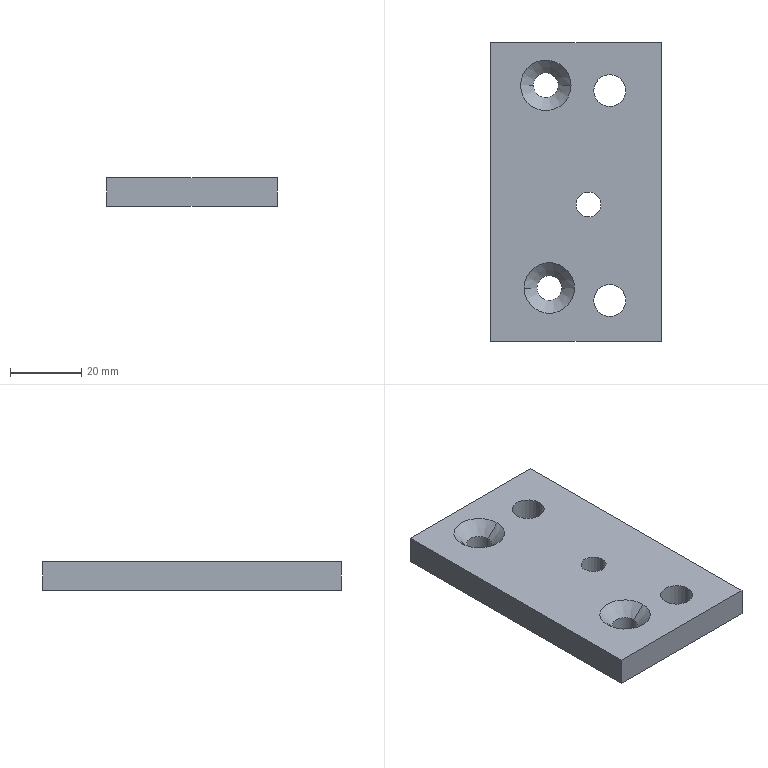Part | 1 solid | 20 faces | box 48 x 84 x 8 mm | volume 29932 mm3 | cylinder 10 | plane 6 | cone 4 | commonest cylinder face diameters 7 x6 9 x4
STEP:
#1=CARTESIAN_POINT('',(0.,0.,0.));
#2=DIRECTION('',(0.,0.,1.));
#3=DIRECTION('',(1.,0.,0.));
#4=AXIS2_PLACEMENT_3D('',#1,#2,#3);
#5=CARTESIAN_POINT('',(-178.858,521.,-248.55));
#6=VERTEX_POINT('',#5);
#7=CARTESIAN_POINT('',(-226.858,521.,-248.55));
#8=VERTEX_POINT('',#7);
#9=CARTESIAN_POINT('',(-178.858,521.,-248.55));
#10=DIRECTION('',(-1.,0.,0.));
#11=VECTOR('',#10,1.);
#12=LINE('',#9,#11);
#13=CARTESIAN_POINT('',(-178.858,521.,-256.55));
#14=DIRECTION('',(0.,1.,0.));
#15=DIRECTION('',(0.,0.,-1.));
#16=AXIS2_PLACEMENT_3D('',#13,#14,#15);
#17=PLANE('',#16);
#18=CARTESIAN_POINT('',(-8.,0.));
#19=DIRECTION('',(0.,1.));
#20=VECTOR('',#19,1.);
#21=LINE('',#18,#20);
#22=(GEOMETRIC_REPRESENTATION_CONTEXT(2)PARAMETRIC_REPRESENTATION_CONTEXT()REPRESENTATION_CONTEXT('',''));
#23=DEFINITIONAL_REPRESENTATION('',(#21),#22);
#24=PCURVE('',#17,#23);
#25=CARTESIAN_POINT('',(-193.358,507.5,-248.55));
#26=DIRECTION('',(0.,0.,1.));
#27=DIRECTION('',(-1.,0.,0.));
#28=AXIS2_PLACEMENT_3D('',#25,#26,#27);
#29=PLANE('',#28);
#30=CARTESIAN_POINT('',(-14.5,-13.5));
#31=DIRECTION('',(1.,0.));
#32=VECTOR('',#31,1.);
#33=LINE('',#30,#32);
#34=(GEOMETRIC_REPRESENTATION_CONTEXT(2)PARAMETRIC_REPRESENTATION_CONTEXT()REPRESENTATION_CONTEXT('',''));
#35=DEFINITIONAL_REPRESENTATION('',(#33),#34);
#36=PCURVE('',#29,#35);
#37=SURFACE_CURVE('',#12,(#24,#36),.PCURVE_S1.);
#38=EDGE_CURVE('',#6,#8,#37,.T.);
#39=ORIENTED_EDGE('',*,*,#38,.F.);
#40=CARTESIAN_POINT('',(-178.858,521.,-256.55));
#41=VERTEX_POINT('',#40);
#42=CARTESIAN_POINT('',(-178.858,521.,-256.55));
#43=DIRECTION('',(0.,0.,1.));
#44=VECTOR('',#43,1.);
#45=LINE('',#42,#44);
#46=CARTESIAN_POINT('',(0.,0.));
#47=DIRECTION('',(-1.,0.));
#48=VECTOR('',#47,1.);
#49=LINE('',#46,#48);
#50=(GEOMETRIC_REPRESENTATION_CONTEXT(2)PARAMETRIC_REPRESENTATION_CONTEXT()REPRESENTATION_CONTEXT('',''));
#51=DEFINITIONAL_REPRESENTATION('',(#49),#50);
#52=PCURVE('',#17,#51);
#53=CARTESIAN_POINT('',(-178.858,437.,-256.55));
#54=DIRECTION('',(1.,0.,0.));
#55=DIRECTION('',(0.,0.,1.));
#56=AXIS2_PLACEMENT_3D('',#53,#54,#55);
#57=PLANE('',#56);
#58=CARTESIAN_POINT('',(0.,-84.));
#59=DIRECTION('',(1.,0.));
#60=VECTOR('',#59,1.);
#61=LINE('',#58,#60);
#62=(GEOMETRIC_REPRESENTATION_CONTEXT(2)PARAMETRIC_REPRESENTATION_CONTEXT()REPRESENTATION_CONTEXT('',''));
#63=DEFINITIONAL_REPRESENTATION('',(#61),#62);
#64=PCURVE('',#57,#63);
#65=SURFACE_CURVE('',#45,(#52,#64),.PCURVE_S1.);
#66=EDGE_CURVE('',#41,#6,#65,.T.);
#67=ORIENTED_EDGE('',*,*,#66,.F.);
#68=CARTESIAN_POINT('',(-226.858,521.,-256.55));
#69=VERTEX_POINT('',#68);
#70=CARTESIAN_POINT('',(-178.858,521.,-256.55));
#71=DIRECTION('',(-1.,0.,0.));
#72=VECTOR('',#71,1.);
#73=LINE('',#70,#72);
#74=CARTESIAN_POINT('',(0.,0.));
#75=DIRECTION('',(0.,1.));
#76=VECTOR('',#75,1.);
#77=LINE('',#74,#76);
#78=(GEOMETRIC_REPRESENTATION_CONTEXT(2)PARAMETRIC_REPRESENTATION_CONTEXT()REPRESENTATION_CONTEXT('',''));
#79=DEFINITIONAL_REPRESENTATION('',(#77),#78);
#80=PCURVE('',#17,#79);
#81=CARTESIAN_POINT('',(-193.358,507.5,-256.55));
#82=DIRECTION('',(0.,0.,1.));
#83=DIRECTION('',(-1.,0.,0.));
#84=AXIS2_PLACEMENT_3D('',#81,#82,#83);
#85=PLANE('',#84);
#86=CARTESIAN_POINT('',(-14.5,-13.5));
#87=DIRECTION('',(1.,0.));
#88=VECTOR('',#87,1.);
#89=LINE('',#86,#88);
#90=(GEOMETRIC_REPRESENTATION_CONTEXT(2)PARAMETRIC_REPRESENTATION_CONTEXT()REPRESENTATION_CONTEXT('',''));
#91=DEFINITIONAL_REPRESENTATION('',(#89),#90);
#92=PCURVE('',#85,#91);
#93=SURFACE_CURVE('',#73,(#80,#92),.PCURVE_S1.);
#94=EDGE_CURVE('',#41,#69,#93,.T.);
#95=ORIENTED_EDGE('',*,*,#94,.T.);
#96=CARTESIAN_POINT('',(-226.858,521.,-256.55));
#97=DIRECTION('',(0.,0.,1.));
#98=VECTOR('',#97,1.);
#99=LINE('',#96,#98);
#100=CARTESIAN_POINT('',(0.,48.));
#101=DIRECTION('',(-1.,0.));
#102=VECTOR('',#101,1.);
#103=LINE('',#100,#102);
#104=(GEOMETRIC_REPRESENTATION_CONTEXT(2)PARAMETRIC_REPRESENTATION_CONTEXT()REPRESENTATION_CONTEXT('',''));
#105=DEFINITIONAL_REPRESENTATION('',(#103),#104);
#106=PCURVE('',#17,#105);
#107=CARTESIAN_POINT('',(-226.858,521.,-256.55));
#108=DIRECTION('',(-1.,0.,0.));
#109=DIRECTION('',(0.,0.,-1.));
#110=AXIS2_PLACEMENT_3D('',#107,#108,#109);
#111=PLANE('',#110);
#112=CARTESIAN_POINT('',(0.,0.));
#113=DIRECTION('',(-1.,0.));
#114=VECTOR('',#113,1.);
#115=LINE('',#112,#114);
#116=(GEOMETRIC_REPRESENTATION_CONTEXT(2)PARAMETRIC_REPRESENTATION_CONTEXT()REPRESENTATION_CONTEXT('',''));
#117=DEFINITIONAL_REPRESENTATION('',(#115),#116);
#118=PCURVE('',#111,#117);
#119=SURFACE_CURVE('',#99,(#106,#118),.PCURVE_S1.);
#120=EDGE_CURVE('',#69,#8,#119,.T.);
#121=ORIENTED_EDGE('',*,*,#120,.T.);
#122=EDGE_LOOP('',(#39,#67,#95,#121));
#123=FACE_BOUND('',#122,.T.);
#124=ADVANCED_FACE('',(#123),#17,.T.);
#125=CARTESIAN_POINT('',(-226.858,437.,-248.55));
#126=VERTEX_POINT('',#125);
#127=CARTESIAN_POINT('',(-226.858,521.,-248.55));
#128=DIRECTION('',(0.,-1.,0.));
#129=VECTOR('',#128,1.);
#130=LINE('',#127,#129);
#131=CARTESIAN_POINT('',(-8.,0.));
#132=DIRECTION('',(0.,1.));
#133=VECTOR('',#132,1.);
#134=LINE('',#131,#133);
#135=(GEOMETRIC_REPRESENTATION_CONTEXT(2)PARAMETRIC_REPRESENTATION_CONTEXT()REPRESENTATION_CONTEXT('',''));
#136=DEFINITIONAL_REPRESENTATION('',(#134),#135);
#137=PCURVE('',#111,#136);
#138=CARTESIAN_POINT('',(33.5,-13.5));
#139=DIRECTION('',(0.,1.));
#140=VECTOR('',#139,1.);
#141=LINE('',#138,#140);
#142=(GEOMETRIC_REPRESENTATION_CONTEXT(2)PARAMETRIC_REPRESENTATION_CONTEXT()REPRESENTATION_CONTEXT('',''));
#143=DEFINITIONAL_REPRESENTATION('',(#141),#142);
#144=PCURVE('',#29,#143);
#145=SURFACE_CURVE('',#130,(#137,#144),.PCURVE_S1.);
#146=EDGE_CURVE('',#8,#126,#145,.T.);
#147=ORIENTED_EDGE('',*,*,#146,.F.);
#148=ORIENTED_EDGE('',*,*,#120,.F.);
#149=CARTESIAN_POINT('',(-226.858,437.,-256.55));
#150=VERTEX_POINT('',#149);
#151=CARTESIAN_POINT('',(-226.858,521.,-256.55));
#152=DIRECTION('',(0.,-1.,0.));
#153=VECTOR('',#152,1.);
#154=LINE('',#151,#153);
#155=CARTESIAN_POINT('',(0.,0.));
#156=DIRECTION('',(0.,1.));
#157=VECTOR('',#156,1.);
#158=LINE('',#155,#157);
#159=(GEOMETRIC_REPRESENTATION_CONTEXT(2)PARAMETRIC_REPRESENTATION_CONTEXT()REPRESENTATION_CONTEXT('',''));
#160=DEFINITIONAL_REPRESENTATION('',(#158),#159);
#161=PCURVE('',#111,#160);
#162=CARTESIAN_POINT('',(33.5,-13.5));
#163=DIRECTION('',(0.,1.));
#164=VECTOR('',#163,1.);
#165=LINE('',#162,#164);
#166=(GEOMETRIC_REPRESENTATION_CONTEXT(2)PARAMETRIC_REPRESENTATION_CONTEXT()REPRESENTATION_CONTEXT('',''));
#167=DEFINITIONAL_REPRESENTATION('',(#165),#166);
#168=PCURVE('',#85,#167);
#169=SURFACE_CURVE('',#154,(#161,#168),.PCURVE_S1.);
#170=EDGE_CURVE('',#69,#150,#169,.T.);
#171=ORIENTED_EDGE('',*,*,#170,.T.);
#172=CARTESIAN_POINT('',(-226.858,437.,-256.55));
#173=DIRECTION('',(0.,0.,1.));
#174=VECTOR('',#173,1.);
#175=LINE('',#172,#174);
#176=CARTESIAN_POINT('',(0.,84.));
#177=DIRECTION('',(-1.,0.));
#178=VECTOR('',#177,1.);
#179=LINE('',#176,#178);
#180=(GEOMETRIC_REPRESENTATION_CONTEXT(2)PARAMETRIC_REPRESENTATION_CONTEXT()REPRESENTATION_CONTEXT('',''));
#181=DEFINITIONAL_REPRESENTATION('',(#179),#180);
#182=PCURVE('',#111,#181);
#183=CARTESIAN_POINT('',(-226.858,437.,-256.55));
#184=DIRECTION('',(0.,-1.,0.));
#185=DIRECTION('',(0.,0.,1.));
#186=AXIS2_PLACEMENT_3D('',#183,#184,#185);
#187=PLANE('',#186);
#188=CARTESIAN_POINT('',(0.,0.));
#189=DIRECTION('',(1.,0.));
#190=VECTOR('',#189,1.);
#191=LINE('',#188,#190);
#192=(GEOMETRIC_REPRESENTATION_CONTEXT(2)PARAMETRIC_REPRESENTATION_CONTEXT()REPRESENTATION_CONTEXT('',''));
#193=DEFINITIONAL_REPRESENTATION('',(#191),#192);
#194=PCURVE('',#187,#193);
#195=SURFACE_CURVE('',#175,(#182,#194),.PCURVE_S1.);
#196=EDGE_CURVE('',#150,#126,#195,.T.);
#197=ORIENTED_EDGE('',*,*,#196,.T.);
#198=EDGE_LOOP('',(#147,#148,#171,#197));
#199=FACE_BOUND('',#198,.T.);
#200=ADVANCED_FACE('',(#199),#111,.T.);
#201=CARTESIAN_POINT('',(-178.858,437.,-248.55));
#202=VERTEX_POINT('',#201);
#203=CARTESIAN_POINT('',(-226.858,437.,-248.55));
#204=DIRECTION('',(1.,0.,0.));
#205=VECTOR('',#204,1.);
#206=LINE('',#203,#205);
#207=CARTESIAN_POINT('',(8.,0.));
#208=DIRECTION('',(0.,-1.));
#209=VECTOR('',#208,1.);
#210=LINE('',#207,#209);
#211=(GEOMETRIC_REPRESENTATION_CONTEXT(2)PARAMETRIC_REPRESENTATION_CONTEXT()REPRESENTATION_CONTEXT('',''));
#212=DEFINITIONAL_REPRESENTATION('',(#210),#211);
#213=PCURVE('',#187,#212);
#214=CARTESIAN_POINT('',(33.5,70.5));
#215=DIRECTION('',(-1.,0.));
#216=VECTOR('',#215,1.);
#217=LINE('',#214,#216);
#218=(GEOMETRIC_REPRESENTATION_CONTEXT(2)PARAMETRIC_REPRESENTATION_CONTEXT()REPRESENTATION_CONTEXT('',''));
#219=DEFINITIONAL_REPRESENTATION('',(#217),#218);
#220=PCURVE('',#29,#219);
#221=SURFACE_CURVE('',#206,(#213,#220),.PCURVE_S1.);
#222=EDGE_CURVE('',#126,#202,#221,.T.);
#223=ORIENTED_EDGE('',*,*,#222,.F.);
#224=ORIENTED_EDGE('',*,*,#196,.F.);
#225=CARTESIAN_POINT('',(-178.858,437.,-256.55));
#226=VERTEX_POINT('',#225);
#227=CARTESIAN_POINT('',(-226.858,437.,-256.55));
#228=DIRECTION('',(1.,0.,0.));
#229=VECTOR('',#228,1.);
#230=LINE('',#227,#229);
#231=CARTESIAN_POINT('',(0.,0.));
#232=DIRECTION('',(0.,-1.));
#233=VECTOR('',#232,1.);
#234=LINE('',#231,#233);
#235=(GEOMETRIC_REPRESENTATION_CONTEXT(2)PARAMETRIC_REPRESENTATION_CONTEXT()REPRESENTATION_CONTEXT('',''));
#236=DEFINITIONAL_REPRESENTATION('',(#234),#235);
#237=PCURVE('',#187,#236);
#238=CARTESIAN_POINT('',(33.5,70.5));
#239=DIRECTION('',(-1.,0.));
#240=VECTOR('',#239,1.);
#241=LINE('',#238,#240);
#242=(GEOMETRIC_REPRESENTATION_CONTEXT(2)PARAMETRIC_REPRESENTATION_CONTEXT()REPRESENTATION_CONTEXT('',''));
#243=DEFINITIONAL_REPRESENTATION('',(#241),#242);
#244=PCURVE('',#85,#243);
#245=SURFACE_CURVE('',#230,(#237,#244),.PCURVE_S1.);
#246=EDGE_CURVE('',#150,#226,#245,.T.);
#247=ORIENTED_EDGE('',*,*,#246,.T.);
#248=CARTESIAN_POINT('',(-178.858,437.,-256.55));
#249=DIRECTION('',(0.,0.,1.));
#250=VECTOR('',#249,1.);
#251=LINE('',#248,#250);
#252=CARTESIAN_POINT('',(0.,-48.));
#253=DIRECTION('',(1.,0.));
#254=VECTOR('',#253,1.);
#255=LINE('',#252,#254);
#256=(GEOMETRIC_REPRESENTATION_CONTEXT(2)PARAMETRIC_REPRESENTATION_CONTEXT()REPRESENTATION_CONTEXT('',''));
#257=DEFINITIONAL_REPRESENTATION('',(#255),#256);
#258=PCURVE('',#187,#257);
#259=CARTESIAN_POINT('',(0.,0.));
#260=DIRECTION('',(1.,0.));
#261=VECTOR('',#260,1.);
#262=LINE('',#259,#261);
#263=(GEOMETRIC_REPRESENTATION_CONTEXT(2)PARAMETRIC_REPRESENTATION_CONTEXT()REPRESENTATION_CONTEXT('',''));
#264=DEFINITIONAL_REPRESENTATION('',(#262),#263);
#265=PCURVE('',#57,#264);
#266=SURFACE_CURVE('',#251,(#258,#265),.PCURVE_S1.);
#267=EDGE_CURVE('',#226,#202,#266,.T.);
#268=ORIENTED_EDGE('',*,*,#267,.T.);
#269=EDGE_LOOP('',(#223,#224,#247,#268));
#270=FACE_BOUND('',#269,.T.);
#271=ADVANCED_FACE('',(#270),#187,.T.);
#272=CARTESIAN_POINT('',(-178.858,437.,-248.55));
#273=DIRECTION('',(0.,1.,0.));
#274=VECTOR('',#273,1.);
#275=LINE('',#272,#274);
#276=CARTESIAN_POINT('',(8.,0.));
#277=DIRECTION('',(0.,-1.));
#278=VECTOR('',#277,1.);
#279=LINE('',#276,#278);
#280=(GEOMETRIC_REPRESENTATION_CONTEXT(2)PARAMETRIC_REPRESENTATION_CONTEXT()REPRESENTATION_CONTEXT('',''));
#281=DEFINITIONAL_REPRESENTATION('',(#279),#280);
#282=PCURVE('',#57,#281);
#283=CARTESIAN_POINT('',(-14.5,70.5));
#284=DIRECTION('',(0.,-1.));
#285=VECTOR('',#284,1.);
#286=LINE('',#283,#285);
#287=(GEOMETRIC_REPRESENTATION_CONTEXT(2)PARAMETRIC_REPRESENTATION_CONTEXT()REPRESENTATION_CONTEXT('',''));
#288=DEFINITIONAL_REPRESENTATION('',(#286),#287);
#289=PCURVE('',#29,#288);
#290=SURFACE_CURVE('',#275,(#282,#289),.PCURVE_S1.);
#291=EDGE_CURVE('',#202,#6,#290,.T.);
#292=ORIENTED_EDGE('',*,*,#291,.F.);
#293=ORIENTED_EDGE('',*,*,#267,.F.);
#294=CARTESIAN_POINT('',(-178.858,437.,-256.55));
#295=DIRECTION('',(0.,1.,0.));
#296=VECTOR('',#295,1.);
#297=LINE('',#294,#296);
#298=CARTESIAN_POINT('',(0.,0.));
#299=DIRECTION('',(0.,-1.));
#300=VECTOR('',#299,1.);
#301=LINE('',#298,#300);
#302=(GEOMETRIC_REPRESENTATION_CONTEXT(2)PARAMETRIC_REPRESENTATION_CONTEXT()REPRESENTATION_CONTEXT('',''));
#303=DEFINITIONAL_REPRESENTATION('',(#301),#302);
#304=PCURVE('',#57,#303);
#305=CARTESIAN_POINT('',(-14.5,70.5));
#306=DIRECTION('',(0.,-1.));
#307=VECTOR('',#306,1.);
#308=LINE('',#305,#307);
#309=(GEOMETRIC_REPRESENTATION_CONTEXT(2)PARAMETRIC_REPRESENTATION_CONTEXT()REPRESENTATION_CONTEXT('',''));
#310=DEFINITIONAL_REPRESENTATION('',(#308),#309);
#311=PCURVE('',#85,#310);
#312=SURFACE_CURVE('',#297,(#304,#311),.PCURVE_S1.);
#313=EDGE_CURVE('',#226,#41,#312,.T.);
#314=ORIENTED_EDGE('',*,*,#313,.T.);
#315=ORIENTED_EDGE('',*,*,#66,.T.);
#316=EDGE_LOOP('',(#292,#293,#314,#315));
#317=FACE_BOUND('',#316,.T.);
#318=ADVANCED_FACE('',(#317),#57,.T.);
#319=CARTESIAN_POINT('',(-206.858,452.,-256.55));
#320=VERTEX_POINT('',#319);
#321=CARTESIAN_POINT('',(-213.858,452.,-256.55));
#322=VERTEX_POINT('',#321);
#323=CARTESIAN_POINT('',(-210.358,452.,-256.55));
#324=DIRECTION('',(0.,0.,1.));
#325=DIRECTION('',(1.,0.,0.));
#326=AXIS2_PLACEMENT_3D('',#323,#324,#325);
#327=CIRCLE('',#326,3.5);
#328=CARTESIAN_POINT('',(17.,55.5));
#329=DIRECTION('',(-1.,0.));
#330=AXIS2_PLACEMENT_2D('',#328,#329);
#331=CIRCLE('',#330,3.5);
#332=(GEOMETRIC_REPRESENTATION_CONTEXT(2)PARAMETRIC_REPRESENTATION_CONTEXT()REPRESENTATION_CONTEXT('',''));
#333=DEFINITIONAL_REPRESENTATION('',(#331),#332);
#334=PCURVE('',#85,#333);
#335=CARTESIAN_POINT('',(-210.358,452.,-298.55));
#336=DIRECTION('',(0.,0.,-1.));
#337=DIRECTION('',(0.,-1.,0.));
#338=AXIS2_PLACEMENT_3D('',#335,#336,#337);
#339=CYLINDRICAL_SURFACE('',#338,3.5);
#340=CARTESIAN_POINT('',(4.712,-42.));
#341=DIRECTION('',(-1.,0.));
#342=VECTOR('',#341,1.);
#343=LINE('',#340,#342);
#344=(GEOMETRIC_REPRESENTATION_CONTEXT(2)PARAMETRIC_REPRESENTATION_CONTEXT()REPRESENTATION_CONTEXT('',''));
#345=DEFINITIONAL_REPRESENTATION('',(#343),#344);
#346=PCURVE('',#339,#345);
#347=SURFACE_CURVE('',#327,(#334,#346),.PCURVE_S1.);
#348=EDGE_CURVE('',#320,#322,#347,.T.);
#349=ORIENTED_EDGE('',*,*,#348,.T.);
#350=CARTESIAN_POINT('',(-210.358,452.,-256.55));
#351=DIRECTION('',(0.,0.,1.));
#352=DIRECTION('',(1.,0.,0.));
#353=AXIS2_PLACEMENT_3D('',#350,#351,#352);
#354=CIRCLE('',#353,3.5);
#355=CARTESIAN_POINT('',(17.,55.5));
#356=DIRECTION('',(-1.,0.));
#357=AXIS2_PLACEMENT_2D('',#355,#356);
#358=CIRCLE('',#357,3.5);
#359=(GEOMETRIC_REPRESENTATION_CONTEXT(2)PARAMETRIC_REPRESENTATION_CONTEXT()REPRESENTATION_CONTEXT('',''));
#360=DEFINITIONAL_REPRESENTATION('',(#358),#359);
#361=PCURVE('',#85,#360);
#362=CARTESIAN_POINT('',(-210.358,452.,-298.55));
#363=DIRECTION('',(0.,0.,-1.));
#364=DIRECTION('',(0.,1.,0.));
#365=AXIS2_PLACEMENT_3D('',#362,#363,#364);
#366=CYLINDRICAL_SURFACE('',#365,3.5);
#367=CARTESIAN_POINT('',(7.854,-42.));
#368=DIRECTION('',(-1.,0.));
#369=VECTOR('',#368,1.);
#370=LINE('',#367,#369);
#371=(GEOMETRIC_REPRESENTATION_CONTEXT(2)PARAMETRIC_REPRESENTATION_CONTEXT()REPRESENTATION_CONTEXT('',''));
#372=DEFINITIONAL_REPRESENTATION('',(#370),#371);
#373=PCURVE('',#366,#372);
#374=SURFACE_CURVE('',#354,(#361,#373),.PCURVE_S1.);
#375=EDGE_CURVE('',#322,#320,#374,.T.);
#376=ORIENTED_EDGE('',*,*,#375,.T.);
#377=EDGE_LOOP('',(#349,#376));
#378=FACE_BOUND('',#377,.T.);
#379=CARTESIAN_POINT('',(-207.858,509.,-256.55));
#380=VERTEX_POINT('',#379);
#381=CARTESIAN_POINT('',(-214.858,509.,-256.55));
#382=VERTEX_POINT('',#381);
#383=CARTESIAN_POINT('',(-211.358,509.,-256.55));
#384=DIRECTION('',(0.,0.,1.));
#385=DIRECTION('',(1.,0.,0.));
#386=AXIS2_PLACEMENT_3D('',#383,#384,#385);
#387=CIRCLE('',#386,3.5);
#388=CARTESIAN_POINT('',(18.,-1.5));
#389=DIRECTION('',(-1.,0.));
#390=AXIS2_PLACEMENT_2D('',#388,#389);
#391=CIRCLE('',#390,3.5);
#392=(GEOMETRIC_REPRESENTATION_CONTEXT(2)PARAMETRIC_REPRESENTATION_CONTEXT()REPRESENTATION_CONTEXT('',''));
#393=DEFINITIONAL_REPRESENTATION('',(#391),#392);
#394=PCURVE('',#85,#393);
#395=CARTESIAN_POINT('',(-211.358,509.,-298.55));
#396=DIRECTION('',(0.,0.,-1.));
#397=DIRECTION('',(0.,-1.,0.));
#398=AXIS2_PLACEMENT_3D('',#395,#396,#397);
#399=CYLINDRICAL_SURFACE('',#398,3.5);
#400=CARTESIAN_POINT('',(4.712,-42.));
#401=DIRECTION('',(-1.,0.));
#402=VECTOR('',#401,1.);
#403=LINE('',#400,#402);
#404=(GEOMETRIC_REPRESENTATION_CONTEXT(2)PARAMETRIC_REPRESENTATION_CONTEXT()REPRESENTATION_CONTEXT('',''));
#405=DEFINITIONAL_REPRESENTATION('',(#403),#404);
#406=PCURVE('',#399,#405);
#407=SURFACE_CURVE('',#387,(#394,#406),.PCURVE_S1.);
#408=EDGE_CURVE('',#380,#382,#407,.T.);
#409=ORIENTED_EDGE('',*,*,#408,.T.);
#410=CARTESIAN_POINT('',(-211.358,509.,-256.55));
#411=DIRECTION('',(0.,0.,1.));
#412=DIRECTION('',(1.,0.,0.));
#413=AXIS2_PLACEMENT_3D('',#410,#411,#412);
#414=CIRCLE('',#413,3.5);
#415=CARTESIAN_POINT('',(18.,-1.5));
#416=DIRECTION('',(-1.,0.));
#417=AXIS2_PLACEMENT_2D('',#415,#416);
#418=CIRCLE('',#417,3.5);
#419=(GEOMETRIC_REPRESENTATION_CONTEXT(2)PARAMETRIC_REPRESENTATION_CONTEXT()REPRESENTATION_CONTEXT('',''));
#420=DEFINITIONAL_REPRESENTATION('',(#418),#419);
#421=PCURVE('',#85,#420);
#422=CARTESIAN_POINT('',(-211.358,509.,-298.55));
#423=DIRECTION('',(0.,0.,-1.));
#424=DIRECTION('',(0.,1.,0.));
#425=AXIS2_PLACEMENT_3D('',#422,#423,#424);
#426=CYLINDRICAL_SURFACE('',#425,3.5);
#427=CARTESIAN_POINT('',(7.854,-42.));
#428=DIRECTION('',(-1.,0.));
#429=VECTOR('',#428,1.);
#430=LINE('',#427,#429);
#431=(GEOMETRIC_REPRESENTATION_CONTEXT(2)PARAMETRIC_REPRESENTATION_CONTEXT()REPRESENTATION_CONTEXT('',''));
#432=DEFINITIONAL_REPRESENTATION('',(#430),#431);
#433=PCURVE('',#426,#432);
#434=SURFACE_CURVE('',#414,(#421,#433),.PCURVE_S1.);
#435=EDGE_CURVE('',#382,#380,#434,.T.);
#436=ORIENTED_EDGE('',*,*,#435,.T.);
#437=EDGE_LOOP('',(#409,#436));
#438=FACE_BOUND('',#437,.T.);
#439=ORIENTED_EDGE('',*,*,#94,.F.);
#440=ORIENTED_EDGE('',*,*,#313,.F.);
#441=ORIENTED_EDGE('',*,*,#246,.F.);
#442=ORIENTED_EDGE('',*,*,#170,.F.);
#443=EDGE_LOOP('',(#439,#440,#441,#442));
#444=FACE_BOUND('',#443,.T.);
#445=CARTESIAN_POINT('',(-197.858,507.5,-256.55));
#446=VERTEX_POINT('',#445);
#447=CARTESIAN_POINT('',(-188.858,507.5,-256.55));
#448=VERTEX_POINT('',#447);
#449=CARTESIAN_POINT('',(-193.358,507.5,-256.55));
#450=DIRECTION('',(0.,0.,1.));
#451=DIRECTION('',(-1.,0.,0.));
#452=AXIS2_PLACEMENT_3D('',#449,#450,#451);
#453=CIRCLE('',#452,4.5);
#454=CARTESIAN_POINT('',(0.,0.));
#455=DIRECTION('',(1.,0.));
#456=AXIS2_PLACEMENT_2D('',#454,#455);
#457=CIRCLE('',#456,4.5);
#458=(GEOMETRIC_REPRESENTATION_CONTEXT(2)PARAMETRIC_REPRESENTATION_CONTEXT()REPRESENTATION_CONTEXT('',''));
#459=DEFINITIONAL_REPRESENTATION('',(#457),#458);
#460=PCURVE('',#85,#459);
#461=CARTESIAN_POINT('',(-193.358,507.5,-256.55));
#462=DIRECTION('',(0.,0.,1.));
#463=DIRECTION('',(0.,1.,0.));
#464=AXIS2_PLACEMENT_3D('',#461,#462,#463);
#465=CYLINDRICAL_SURFACE('',#464,4.5);
#466=CARTESIAN_POINT('',(1.571,0.));
#467=DIRECTION('',(1.,0.));
#468=VECTOR('',#467,1.);
#469=LINE('',#466,#468);
#470=(GEOMETRIC_REPRESENTATION_CONTEXT(2)PARAMETRIC_REPRESENTATION_CONTEXT()REPRESENTATION_CONTEXT('',''));
#471=DEFINITIONAL_REPRESENTATION('',(#469),#470);
#472=PCURVE('',#465,#471);
#473=SURFACE_CURVE('',#453,(#460,#472),.PCURVE_S1.);
#474=EDGE_CURVE('',#446,#448,#473,.T.);
#475=ORIENTED_EDGE('',*,*,#474,.T.);
#476=CARTESIAN_POINT('',(-193.358,507.5,-256.55));
#477=DIRECTION('',(0.,0.,1.));
#478=DIRECTION('',(-1.,0.,0.));
#479=AXIS2_PLACEMENT_3D('',#476,#477,#478);
#480=CIRCLE('',#479,4.5);
#481=CARTESIAN_POINT('',(0.,0.));
#482=DIRECTION('',(1.,0.));
#483=AXIS2_PLACEMENT_2D('',#481,#482);
#484=CIRCLE('',#483,4.5);
#485=(GEOMETRIC_REPRESENTATION_CONTEXT(2)PARAMETRIC_REPRESENTATION_CONTEXT()REPRESENTATION_CONTEXT('',''));
#486=DEFINITIONAL_REPRESENTATION('',(#484),#485);
#487=PCURVE('',#85,#486);
#488=CARTESIAN_POINT('',(-193.358,507.5,-256.55));
#489=DIRECTION('',(0.,0.,1.));
#490=DIRECTION('',(0.,-1.,0.));
#491=AXIS2_PLACEMENT_3D('',#488,#489,#490);
#492=CYLINDRICAL_SURFACE('',#491,4.5);
#493=CARTESIAN_POINT('',(-1.571,0.));
#494=DIRECTION('',(1.,0.));
#495=VECTOR('',#494,1.);
#496=LINE('',#493,#495);
#497=(GEOMETRIC_REPRESENTATION_CONTEXT(2)PARAMETRIC_REPRESENTATION_CONTEXT()REPRESENTATION_CONTEXT('',''));
#498=DEFINITIONAL_REPRESENTATION('',(#496),#497);
#499=PCURVE('',#492,#498);
#500=SURFACE_CURVE('',#480,(#487,#499),.PCURVE_S1.);
#501=EDGE_CURVE('',#448,#446,#500,.T.);
#502=ORIENTED_EDGE('',*,*,#501,.T.);
#503=EDGE_LOOP('',(#475,#502));
#504=FACE_BOUND('',#503,.T.);
#505=CARTESIAN_POINT('',(-202.858,475.5,-256.55));
#506=VERTEX_POINT('',#505);
#507=CARTESIAN_POINT('',(-195.858,475.5,-256.55));
#508=VERTEX_POINT('',#507);
#509=CARTESIAN_POINT('',(-199.358,475.5,-256.55));
#510=DIRECTION('',(0.,0.,1.));
#511=DIRECTION('',(-1.,0.,0.));
#512=AXIS2_PLACEMENT_3D('',#509,#510,#511);
#513=CIRCLE('',#512,3.5);
#514=CARTESIAN_POINT('',(6.,32.));
#515=DIRECTION('',(1.,0.));
#516=AXIS2_PLACEMENT_2D('',#514,#515);
#517=CIRCLE('',#516,3.5);
#518=(GEOMETRIC_REPRESENTATION_CONTEXT(2)PARAMETRIC_REPRESENTATION_CONTEXT()REPRESENTATION_CONTEXT('',''));
#519=DEFINITIONAL_REPRESENTATION('',(#517),#518);
#520=PCURVE('',#85,#519);
#521=CARTESIAN_POINT('',(-199.358,475.5,-256.55));
#522=DIRECTION('',(0.,0.,1.));
#523=DIRECTION('',(0.,1.,0.));
#524=AXIS2_PLACEMENT_3D('',#521,#522,#523);
#525=CYLINDRICAL_SURFACE('',#524,3.5);
#526=CARTESIAN_POINT('',(1.571,0.));
#527=DIRECTION('',(1.,0.));
#528=VECTOR('',#527,1.);
#529=LINE('',#526,#528);
#530=(GEOMETRIC_REPRESENTATION_CONTEXT(2)PARAMETRIC_REPRESENTATION_CONTEXT()REPRESENTATION_CONTEXT('',''));
#531=DEFINITIONAL_REPRESENTATION('',(#529),#530);
#532=PCURVE('',#525,#531);
#533=SURFACE_CURVE('',#513,(#520,#532),.PCURVE_S1.);
#534=EDGE_CURVE('',#506,#508,#533,.T.);
#535=ORIENTED_EDGE('',*,*,#534,.T.);
#536=CARTESIAN_POINT('',(-199.358,475.5,-256.55));
#537=DIRECTION('',(0.,0.,1.));
#538=DIRECTION('',(-1.,0.,0.));
#539=AXIS2_PLACEMENT_3D('',#536,#537,#538);
#540=CIRCLE('',#539,3.5);
#541=CARTESIAN_POINT('',(6.,32.));
#542=DIRECTION('',(1.,0.));
#543=AXIS2_PLACEMENT_2D('',#541,#542);
#544=CIRCLE('',#543,3.5);
#545=(GEOMETRIC_REPRESENTATION_CONTEXT(2)PARAMETRIC_REPRESENTATION_CONTEXT()REPRESENTATION_CONTEXT('',''));
#546=DEFINITIONAL_REPRESENTATION('',(#544),#545);
#547=PCURVE('',#85,#546);
#548=CARTESIAN_POINT('',(-199.358,475.5,-256.55));
#549=DIRECTION('',(0.,0.,1.));
#550=DIRECTION('',(0.,-1.,0.));
#551=AXIS2_PLACEMENT_3D('',#548,#549,#550);
#552=CYLINDRICAL_SURFACE('',#551,3.5);
#553=CARTESIAN_POINT('',(-1.571,0.));
#554=DIRECTION('',(1.,0.));
#555=VECTOR('',#554,1.);
#556=LINE('',#553,#555);
#557=(GEOMETRIC_REPRESENTATION_CONTEXT(2)PARAMETRIC_REPRESENTATION_CONTEXT()REPRESENTATION_CONTEXT('',''));
#558=DEFINITIONAL_REPRESENTATION('',(#556),#557);
#559=PCURVE('',#552,#558);
#560=SURFACE_CURVE('',#540,(#547,#559),.PCURVE_S1.);
#561=EDGE_CURVE('',#508,#506,#560,.T.);
#562=ORIENTED_EDGE('',*,*,#561,.T.);
#563=EDGE_LOOP('',(#535,#562));
#564=FACE_BOUND('',#563,.T.);
#565=CARTESIAN_POINT('',(-197.858,448.5,-256.55));
#566=VERTEX_POINT('',#565);
#567=CARTESIAN_POINT('',(-188.858,448.5,-256.55));
#568=VERTEX_POINT('',#567);
#569=CARTESIAN_POINT('',(-193.358,448.5,-256.55));
#570=DIRECTION('',(0.,0.,1.));
#571=DIRECTION('',(-1.,0.,0.));
#572=AXIS2_PLACEMENT_3D('',#569,#570,#571);
#573=CIRCLE('',#572,4.5);
#574=CARTESIAN_POINT('',(0.,59.));
#575=DIRECTION('',(1.,0.));
#576=AXIS2_PLACEMENT_2D('',#574,#575);
#577=CIRCLE('',#576,4.5);
#578=(GEOMETRIC_REPRESENTATION_CONTEXT(2)PARAMETRIC_REPRESENTATION_CONTEXT()REPRESENTATION_CONTEXT('',''));
#579=DEFINITIONAL_REPRESENTATION('',(#577),#578);
#580=PCURVE('',#85,#579);
#581=CARTESIAN_POINT('',(-193.358,448.5,-256.55));
#582=DIRECTION('',(0.,0.,1.));
#583=DIRECTION('',(0.,1.,0.));
#584=AXIS2_PLACEMENT_3D('',#581,#582,#583);
#585=CYLINDRICAL_SURFACE('',#584,4.5);
#586=CARTESIAN_POINT('',(1.571,0.));
#587=DIRECTION('',(1.,0.));
#588=VECTOR('',#587,1.);
#589=LINE('',#586,#588);
#590=(GEOMETRIC_REPRESENTATION_CONTEXT(2)PARAMETRIC_REPRESENTATION_CONTEXT()REPRESENTATION_CONTEXT('',''));
#591=DEFINITIONAL_REPRESENTATION('',(#589),#590);
#592=PCURVE('',#585,#591);
#593=SURFACE_CURVE('',#573,(#580,#592),.PCURVE_S1.);
#594=EDGE_CURVE('',#566,#568,#593,.T.);
#595=ORIENTED_EDGE('',*,*,#594,.T.);
#596=CARTESIAN_POINT('',(-193.358,448.5,-256.55));
#597=DIRECTION('',(0.,0.,1.));
#598=DIRECTION('',(-1.,0.,0.));
#599=AXIS2_PLACEMENT_3D('',#596,#597,#598);
#600=CIRCLE('',#599,4.5);
#601=CARTESIAN_POINT('',(0.,59.));
#602=DIRECTION('',(1.,0.));
#603=AXIS2_PLACEMENT_2D('',#601,#602);
#604=CIRCLE('',#603,4.5);
#605=(GEOMETRIC_REPRESENTATION_CONTEXT(2)PARAMETRIC_REPRESENTATION_CONTEXT()REPRESENTATION_CONTEXT('',''));
#606=DEFINITIONAL_REPRESENTATION('',(#604),#605);
#607=PCURVE('',#85,#606);
#608=CARTESIAN_POINT('',(-193.358,448.5,-256.55));
#609=DIRECTION('',(0.,0.,1.));
#610=DIRECTION('',(0.,-1.,0.));
#611=AXIS2_PLACEMENT_3D('',#608,#609,#610);
#612=CYLINDRICAL_SURFACE('',#611,4.5);
#613=CARTESIAN_POINT('',(-1.571,0.));
#614=DIRECTION('',(1.,0.));
#615=VECTOR('',#614,1.);
#616=LINE('',#613,#615);
#617=(GEOMETRIC_REPRESENTATION_CONTEXT(2)PARAMETRIC_REPRESENTATION_CONTEXT()REPRESENTATION_CONTEXT('',''));
#618=DEFINITIONAL_REPRESENTATION('',(#616),#617);
#619=PCURVE('',#612,#618);
#620=SURFACE_CURVE('',#600,(#607,#619),.PCURVE_S1.);
#621=EDGE_CURVE('',#568,#566,#620,.T.);
#622=ORIENTED_EDGE('',*,*,#621,.T.);
#623=EDGE_LOOP('',(#595,#622));
#624=FACE_BOUND('',#623,.T.);
#625=ADVANCED_FACE('',(#378,#438,#444,#504,#564,#624),#85,.F.);
#626=ORIENTED_EDGE('',*,*,#621,.T.);
#627=CARTESIAN_POINT('',(-197.858,448.5,-248.55));
#628=VERTEX_POINT('',#627);
#629=CARTESIAN_POINT('',(-197.858,448.5,-256.55));
#630=DIRECTION('',(0.,0.,1.));
#631=VECTOR('',#630,1.);
#632=LINE('',#629,#631);
#633=CARTESIAN_POINT('',(4.712,0.));
#634=DIRECTION('',(0.,1.));
#635=VECTOR('',#634,1.);
#636=LINE('',#633,#635);
#637=(GEOMETRIC_REPRESENTATION_CONTEXT(2)PARAMETRIC_REPRESENTATION_CONTEXT()REPRESENTATION_CONTEXT('',''));
#638=DEFINITIONAL_REPRESENTATION('',(#636),#637);
#639=PCURVE('',#612,#638);
#640=CARTESIAN_POINT('',(1.571,0.));
#641=DIRECTION('',(0.,1.));
#642=VECTOR('',#641,1.);
#643=LINE('',#640,#642);
#644=(GEOMETRIC_REPRESENTATION_CONTEXT(2)PARAMETRIC_REPRESENTATION_CONTEXT()REPRESENTATION_CONTEXT('',''));
#645=DEFINITIONAL_REPRESENTATION('',(#643),#644);
#646=PCURVE('',#585,#645);
#647=SURFACE_CURVE('',#632,(#639,#646),.PCURVE_S1.);
#648=EDGE_CURVE('',#566,#628,#647,.T.);
#649=ORIENTED_EDGE('',*,*,#648,.T.);
#650=CARTESIAN_POINT('',(-188.858,448.5,-248.55));
#651=VERTEX_POINT('',#650);
#652=CARTESIAN_POINT('',(-193.358,448.5,-248.55));
#653=DIRECTION('',(0.,0.,1.));
#654=DIRECTION('',(-1.,0.,0.));
#655=AXIS2_PLACEMENT_3D('',#652,#653,#654);
#656=CIRCLE('',#655,4.5);
#657=CARTESIAN_POINT('',(-1.571,8.));
#658=DIRECTION('',(1.,0.));
#659=VECTOR('',#658,1.);
#660=LINE('',#657,#659);
#661=(GEOMETRIC_REPRESENTATION_CONTEXT(2)PARAMETRIC_REPRESENTATION_CONTEXT()REPRESENTATION_CONTEXT('',''));
#662=DEFINITIONAL_REPRESENTATION('',(#660),#661);
#663=PCURVE('',#612,#662);
#664=CARTESIAN_POINT('',(0.,59.));
#665=DIRECTION('',(1.,0.));
#666=AXIS2_PLACEMENT_2D('',#664,#665);
#667=CIRCLE('',#666,4.5);
#668=(GEOMETRIC_REPRESENTATION_CONTEXT(2)PARAMETRIC_REPRESENTATION_CONTEXT()REPRESENTATION_CONTEXT('',''));
#669=DEFINITIONAL_REPRESENTATION('',(#667),#668);
#670=PCURVE('',#29,#669);
#671=SURFACE_CURVE('',#656,(#663,#670),.PCURVE_S1.);
#672=EDGE_CURVE('',#651,#628,#671,.T.);
#673=ORIENTED_EDGE('',*,*,#672,.F.);
#674=CARTESIAN_POINT('',(-188.858,448.5,-256.55));
#675=DIRECTION('',(0.,0.,1.));
#676=VECTOR('',#675,1.);
#677=LINE('',#674,#676);
#678=CARTESIAN_POINT('',(1.571,0.));
#679=DIRECTION('',(0.,1.));
#680=VECTOR('',#679,1.);
#681=LINE('',#678,#680);
#682=(GEOMETRIC_REPRESENTATION_CONTEXT(2)PARAMETRIC_REPRESENTATION_CONTEXT()REPRESENTATION_CONTEXT('',''));
#683=DEFINITIONAL_REPRESENTATION('',(#681),#682);
#684=PCURVE('',#612,#683);
#685=CARTESIAN_POINT('',(4.712,0.));
#686=DIRECTION('',(0.,1.));
#687=VECTOR('',#686,1.);
#688=LINE('',#685,#687);
#689=(GEOMETRIC_REPRESENTATION_CONTEXT(2)PARAMETRIC_REPRESENTATION_CONTEXT()REPRESENTATION_CONTEXT('',''));
#690=DEFINITIONAL_REPRESENTATION('',(#688),#689);
#691=PCURVE('',#585,#690);
#692=SURFACE_CURVE('',#677,(#684,#691),.PCURVE_S1.);
#693=EDGE_CURVE('',#568,#651,#692,.T.);
#694=ORIENTED_EDGE('',*,*,#693,.F.);
#695=EDGE_LOOP('',(#626,#649,#673,#694));
#696=FACE_BOUND('',#695,.F.);
#697=ADVANCED_FACE('',(#696),#612,.F.);
#698=CARTESIAN_POINT('',(-217.458,452.,-248.55));
#699=VERTEX_POINT('',#698);
#700=CARTESIAN_POINT('',(-203.258,452.,-248.55));
#701=VERTEX_POINT('',#700);
#702=CARTESIAN_POINT('',(-210.358,452.,-248.55));
#703=DIRECTION('',(0.,0.,-1.));
#704=DIRECTION('',(-1.,0.,0.));
#705=AXIS2_PLACEMENT_3D('',#702,#703,#704);
#706=CIRCLE('',#705,7.1);
#707=CARTESIAN_POINT('',(24.1,55.5));
#708=CARTESIAN_POINT('',(24.1,43.203));
#709=CARTESIAN_POINT('',(13.45,49.351));
#710=CARTESIAN_POINT('',(2.8,55.5));
#711=CARTESIAN_POINT('',(13.45,61.649));
#712=CARTESIAN_POINT('',(24.1,67.798));
#713=CARTESIAN_POINT('',(24.1,55.5));
#714=(BOUNDED_CURVE()B_SPLINE_CURVE(2,(#707,#708,#709,#710,#711,#712,#713),.UNSPECIFIED.,.T.,.F.)B_SPLINE_CURVE_WITH_KNOTS((1,2,2,2,2,1),(-2.094,0.,2.094,4.189,6.283,8.378),.UNSPECIFIED.)CURVE()GEOMETRIC_REPRESENTATION_ITEM()RATIONAL_B_SPLINE_CURVE((1.,0.5,1.,0.5,1.,0.5,1.))REPRESENTATION_ITEM(''));
#715=(GEOMETRIC_REPRESENTATION_CONTEXT(2)PARAMETRIC_REPRESENTATION_CONTEXT()REPRESENTATION_CONTEXT('',''));
#716=DEFINITIONAL_REPRESENTATION('',(#714),#715);
#717=PCURVE('',#29,#716);
#718=CARTESIAN_POINT('',(-210.358,452.,-248.55));
#719=DIRECTION('',(0.,0.,1.));
#720=DIRECTION('',(0.,-1.,0.));
#721=AXIS2_PLACEMENT_3D('',#718,#719,#720);
#722=CONICAL_SURFACE('',#721,7.1,0.7854);
#723=CARTESIAN_POINT('',(4.712,0.));
#724=DIRECTION('',(-1.,0.));
#725=VECTOR('',#724,1.);
#726=LINE('',#723,#725);
#727=(GEOMETRIC_REPRESENTATION_CONTEXT(2)PARAMETRIC_REPRESENTATION_CONTEXT()REPRESENTATION_CONTEXT('',''));
#728=DEFINITIONAL_REPRESENTATION('',(#726),#727);
#729=PCURVE('',#722,#728);
#730=SURFACE_CURVE('',#706,(#717,#729),.PCURVE_S1.);
#731=EDGE_CURVE('',#699,#701,#730,.T.);
#732=ORIENTED_EDGE('',*,*,#731,.T.);
#733=CARTESIAN_POINT('',(-210.358,452.,-248.55));
#734=DIRECTION('',(0.,0.,-1.));
#735=DIRECTION('',(-1.,0.,0.));
#736=AXIS2_PLACEMENT_3D('',#733,#734,#735);
#737=CIRCLE('',#736,7.1);
#738=CARTESIAN_POINT('',(24.1,55.5));
#739=CARTESIAN_POINT('',(24.1,43.203));
#740=CARTESIAN_POINT('',(13.45,49.351));
#741=CARTESIAN_POINT('',(2.8,55.5));
#742=CARTESIAN_POINT('',(13.45,61.649));
#743=CARTESIAN_POINT('',(24.1,67.798));
#744=CARTESIAN_POINT('',(24.1,55.5));
#745=(BOUNDED_CURVE()B_SPLINE_CURVE(2,(#738,#739,#740,#741,#742,#743,#744),.UNSPECIFIED.,.T.,.F.)B_SPLINE_CURVE_WITH_KNOTS((1,2,2,2,2,1),(-2.094,0.,2.094,4.189,6.283,8.378),.UNSPECIFIED.)CURVE()GEOMETRIC_REPRESENTATION_ITEM()RATIONAL_B_SPLINE_CURVE((1.,0.5,1.,0.5,1.,0.5,1.))REPRESENTATION_ITEM(''));
#746=(GEOMETRIC_REPRESENTATION_CONTEXT(2)PARAMETRIC_REPRESENTATION_CONTEXT()REPRESENTATION_CONTEXT('',''));
#747=DEFINITIONAL_REPRESENTATION('',(#745),#746);
#748=PCURVE('',#29,#747);
#749=CARTESIAN_POINT('',(-210.358,452.,-248.55));
#750=DIRECTION('',(0.,0.,1.));
#751=DIRECTION('',(0.,1.,0.));
#752=AXIS2_PLACEMENT_3D('',#749,#750,#751);
#753=CONICAL_SURFACE('',#752,7.1,0.7854);
#754=CARTESIAN_POINT('',(7.854,0.));
#755=DIRECTION('',(-1.,0.));
#756=VECTOR('',#755,1.);
#757=LINE('',#754,#756);
#758=(GEOMETRIC_REPRESENTATION_CONTEXT(2)PARAMETRIC_REPRESENTATION_CONTEXT()REPRESENTATION_CONTEXT('',''));
#759=DEFINITIONAL_REPRESENTATION('',(#757),#758);
#760=PCURVE('',#753,#759);
#761=SURFACE_CURVE('',#737,(#748,#760),.PCURVE_S1.);
#762=EDGE_CURVE('',#701,#699,#761,.T.);
#763=ORIENTED_EDGE('',*,*,#762,.T.);
#764=EDGE_LOOP('',(#732,#763));
#765=FACE_BOUND('',#764,.T.);
#766=CARTESIAN_POINT('',(-218.458,509.,-248.55));
#767=VERTEX_POINT('',#766);
#768=CARTESIAN_POINT('',(-204.258,509.,-248.55));
#769=VERTEX_POINT('',#768);
#770=CARTESIAN_POINT('',(-211.358,509.,-248.55));
#771=DIRECTION('',(0.,0.,-1.));
#772=DIRECTION('',(-1.,0.,0.));
#773=AXIS2_PLACEMENT_3D('',#770,#771,#772);
#774=CIRCLE('',#773,7.1);
#775=CARTESIAN_POINT('',(25.1,-1.5));
#776=CARTESIAN_POINT('',(25.1,-13.798));
#777=CARTESIAN_POINT('',(14.45,-7.649));
#778=CARTESIAN_POINT('',(3.8,-1.5));
#779=CARTESIAN_POINT('',(14.45,4.649));
#780=CARTESIAN_POINT('',(25.1,10.798));
#781=CARTESIAN_POINT('',(25.1,-1.5));
#782=(BOUNDED_CURVE()B_SPLINE_CURVE(2,(#775,#776,#777,#778,#779,#780,#781),.UNSPECIFIED.,.T.,.F.)B_SPLINE_CURVE_WITH_KNOTS((1,2,2,2,2,1),(-2.094,0.,2.094,4.189,6.283,8.378),.UNSPECIFIED.)CURVE()GEOMETRIC_REPRESENTATION_ITEM()RATIONAL_B_SPLINE_CURVE((1.,0.5,1.,0.5,1.,0.5,1.))REPRESENTATION_ITEM(''));
#783=(GEOMETRIC_REPRESENTATION_CONTEXT(2)PARAMETRIC_REPRESENTATION_CONTEXT()REPRESENTATION_CONTEXT('',''));
#784=DEFINITIONAL_REPRESENTATION('',(#782),#783);
#785=PCURVE('',#29,#784);
#786=CARTESIAN_POINT('',(-211.358,509.,-248.55));
#787=DIRECTION('',(0.,0.,1.));
#788=DIRECTION('',(0.,-1.,0.));
#789=AXIS2_PLACEMENT_3D('',#786,#787,#788);
#790=CONICAL_SURFACE('',#789,7.1,0.7854);
#791=CARTESIAN_POINT('',(4.712,0.));
#792=DIRECTION('',(-1.,0.));
#793=VECTOR('',#792,1.);
#794=LINE('',#791,#793);
#795=(GEOMETRIC_REPRESENTATION_CONTEXT(2)PARAMETRIC_REPRESENTATION_CONTEXT()REPRESENTATION_CONTEXT('',''));
#796=DEFINITIONAL_REPRESENTATION('',(#794),#795);
#797=PCURVE('',#790,#796);
#798=SURFACE_CURVE('',#774,(#785,#797),.PCURVE_S1.);
#799=EDGE_CURVE('',#767,#769,#798,.T.);
#800=ORIENTED_EDGE('',*,*,#799,.T.);
#801=CARTESIAN_POINT('',(-211.358,509.,-248.55));
#802=DIRECTION('',(0.,0.,-1.));
#803=DIRECTION('',(-1.,0.,0.));
#804=AXIS2_PLACEMENT_3D('',#801,#802,#803);
#805=CIRCLE('',#804,7.1);
#806=CARTESIAN_POINT('',(25.1,-1.5));
#807=CARTESIAN_POINT('',(25.1,-13.798));
#808=CARTESIAN_POINT('',(14.45,-7.649));
#809=CARTESIAN_POINT('',(3.8,-1.5));
#810=CARTESIAN_POINT('',(14.45,4.649));
#811=CARTESIAN_POINT('',(25.1,10.798));
#812=CARTESIAN_POINT('',(25.1,-1.5));
#813=(BOUNDED_CURVE()B_SPLINE_CURVE(2,(#806,#807,#808,#809,#810,#811,#812),.UNSPECIFIED.,.T.,.F.)B_SPLINE_CURVE_WITH_KNOTS((1,2,2,2,2,1),(-2.094,0.,2.094,4.189,6.283,8.378),.UNSPECIFIED.)CURVE()GEOMETRIC_REPRESENTATION_ITEM()RATIONAL_B_SPLINE_CURVE((1.,0.5,1.,0.5,1.,0.5,1.))REPRESENTATION_ITEM(''));
#814=(GEOMETRIC_REPRESENTATION_CONTEXT(2)PARAMETRIC_REPRESENTATION_CONTEXT()REPRESENTATION_CONTEXT('',''));
#815=DEFINITIONAL_REPRESENTATION('',(#813),#814);
#816=PCURVE('',#29,#815);
#817=CARTESIAN_POINT('',(-211.358,509.,-248.55));
#818=DIRECTION('',(0.,0.,1.));
#819=DIRECTION('',(0.,1.,0.));
#820=AXIS2_PLACEMENT_3D('',#817,#818,#819);
#821=CONICAL_SURFACE('',#820,7.1,0.7854);
#822=CARTESIAN_POINT('',(7.854,0.));
#823=DIRECTION('',(-1.,0.));
#824=VECTOR('',#823,1.);
#825=LINE('',#822,#824);
#826=(GEOMETRIC_REPRESENTATION_CONTEXT(2)PARAMETRIC_REPRESENTATION_CONTEXT()REPRESENTATION_CONTEXT('',''));
#827=DEFINITIONAL_REPRESENTATION('',(#825),#826);
#828=PCURVE('',#821,#827);
#829=SURFACE_CURVE('',#805,(#816,#828),.PCURVE_S1.);
#830=EDGE_CURVE('',#769,#767,#829,.T.);
#831=ORIENTED_EDGE('',*,*,#830,.T.);
#832=EDGE_LOOP('',(#800,#831));
#833=FACE_BOUND('',#832,.T.);
#834=ORIENTED_EDGE('',*,*,#38,.T.);
#835=ORIENTED_EDGE('',*,*,#146,.T.);
#836=ORIENTED_EDGE('',*,*,#222,.T.);
#837=ORIENTED_EDGE('',*,*,#291,.T.);
#838=EDGE_LOOP('',(#834,#835,#836,#837));
#839=FACE_BOUND('',#838,.T.);
#840=CARTESIAN_POINT('',(-188.858,507.5,-248.55));
#841=VERTEX_POINT('',#840);
#842=CARTESIAN_POINT('',(-197.858,507.5,-248.55));
#843=VERTEX_POINT('',#842);
#844=CARTESIAN_POINT('',(-193.358,507.5,-248.55));
#845=DIRECTION('',(0.,0.,1.));
#846=DIRECTION('',(-1.,0.,0.));
#847=AXIS2_PLACEMENT_3D('',#844,#845,#846);
#848=CIRCLE('',#847,4.5);
#849=CARTESIAN_POINT('',(0.,0.));
#850=DIRECTION('',(1.,0.));
#851=AXIS2_PLACEMENT_2D('',#849,#850);
#852=CIRCLE('',#851,4.5);
#853=(GEOMETRIC_REPRESENTATION_CONTEXT(2)PARAMETRIC_REPRESENTATION_CONTEXT()REPRESENTATION_CONTEXT('',''));
#854=DEFINITIONAL_REPRESENTATION('',(#852),#853);
#855=PCURVE('',#29,#854);
#856=CARTESIAN_POINT('',(-1.571,8.));
#857=DIRECTION('',(1.,0.));
#858=VECTOR('',#857,1.);
#859=LINE('',#856,#858);
#860=(GEOMETRIC_REPRESENTATION_CONTEXT(2)PARAMETRIC_REPRESENTATION_CONTEXT()REPRESENTATION_CONTEXT('',''));
#861=DEFINITIONAL_REPRESENTATION('',(#859),#860);
#862=PCURVE('',#492,#861);
#863=SURFACE_CURVE('',#848,(#855,#862),.PCURVE_S1.);
#864=EDGE_CURVE('',#841,#843,#863,.T.);
#865=ORIENTED_EDGE('',*,*,#864,.F.);
#866=CARTESIAN_POINT('',(-193.358,507.5,-248.55));
#867=DIRECTION('',(0.,0.,1.));
#868=DIRECTION('',(-1.,0.,0.));
#869=AXIS2_PLACEMENT_3D('',#866,#867,#868);
#870=CIRCLE('',#869,4.5);
#871=CARTESIAN_POINT('',(0.,0.));
#872=DIRECTION('',(1.,0.));
#873=AXIS2_PLACEMENT_2D('',#871,#872);
#874=CIRCLE('',#873,4.5);
#875=(GEOMETRIC_REPRESENTATION_CONTEXT(2)PARAMETRIC_REPRESENTATION_CONTEXT()REPRESENTATION_CONTEXT('',''));
#876=DEFINITIONAL_REPRESENTATION('',(#874),#875);
#877=PCURVE('',#29,#876);
#878=CARTESIAN_POINT('',(1.571,8.));
#879=DIRECTION('',(1.,0.));
#880=VECTOR('',#879,1.);
#881=LINE('',#878,#880);
#882=(GEOMETRIC_REPRESENTATION_CONTEXT(2)PARAMETRIC_REPRESENTATION_CONTEXT()REPRESENTATION_CONTEXT('',''));
#883=DEFINITIONAL_REPRESENTATION('',(#881),#882);
#884=PCURVE('',#465,#883);
#885=SURFACE_CURVE('',#870,(#877,#884),.PCURVE_S1.);
#886=EDGE_CURVE('',#843,#841,#885,.T.);
#887=ORIENTED_EDGE('',*,*,#886,.F.);
#888=EDGE_LOOP('',(#865,#887));
#889=FACE_BOUND('',#888,.T.);
#890=CARTESIAN_POINT('',(-195.858,475.5,-248.55));
#891=VERTEX_POINT('',#890);
#892=CARTESIAN_POINT('',(-202.858,475.5,-248.55));
#893=VERTEX_POINT('',#892);
#894=CARTESIAN_POINT('',(-199.358,475.5,-248.55));
#895=DIRECTION('',(0.,0.,1.));
#896=DIRECTION('',(-1.,0.,0.));
#897=AXIS2_PLACEMENT_3D('',#894,#895,#896);
#898=CIRCLE('',#897,3.5);
#899=CARTESIAN_POINT('',(6.,32.));
#900=DIRECTION('',(1.,0.));
#901=AXIS2_PLACEMENT_2D('',#899,#900);
#902=CIRCLE('',#901,3.5);
#903=(GEOMETRIC_REPRESENTATION_CONTEXT(2)PARAMETRIC_REPRESENTATION_CONTEXT()REPRESENTATION_CONTEXT('',''));
#904=DEFINITIONAL_REPRESENTATION('',(#902),#903);
#905=PCURVE('',#29,#904);
#906=CARTESIAN_POINT('',(-1.571,8.));
#907=DIRECTION('',(1.,0.));
#908=VECTOR('',#907,1.);
#909=LINE('',#906,#908);
#910=(GEOMETRIC_REPRESENTATION_CONTEXT(2)PARAMETRIC_REPRESENTATION_CONTEXT()REPRESENTATION_CONTEXT('',''));
#911=DEFINITIONAL_REPRESENTATION('',(#909),#910);
#912=PCURVE('',#552,#911);
#913=SURFACE_CURVE('',#898,(#905,#912),.PCURVE_S1.);
#914=EDGE_CURVE('',#891,#893,#913,.T.);
#915=ORIENTED_EDGE('',*,*,#914,.F.);
#916=CARTESIAN_POINT('',(-199.358,475.5,-248.55));
#917=DIRECTION('',(0.,0.,1.));
#918=DIRECTION('',(-1.,0.,0.));
#919=AXIS2_PLACEMENT_3D('',#916,#917,#918);
#920=CIRCLE('',#919,3.5);
#921=CARTESIAN_POINT('',(6.,32.));
#922=DIRECTION('',(1.,0.));
#923=AXIS2_PLACEMENT_2D('',#921,#922);
#924=CIRCLE('',#923,3.5);
#925=(GEOMETRIC_REPRESENTATION_CONTEXT(2)PARAMETRIC_REPRESENTATION_CONTEXT()REPRESENTATION_CONTEXT('',''));
#926=DEFINITIONAL_REPRESENTATION('',(#924),#925);
#927=PCURVE('',#29,#926);
#928=CARTESIAN_POINT('',(1.571,8.));
#929=DIRECTION('',(1.,0.));
#930=VECTOR('',#929,1.);
#931=LINE('',#928,#930);
#932=(GEOMETRIC_REPRESENTATION_CONTEXT(2)PARAMETRIC_REPRESENTATION_CONTEXT()REPRESENTATION_CONTEXT('',''));
#933=DEFINITIONAL_REPRESENTATION('',(#931),#932);
#934=PCURVE('',#525,#933);
#935=SURFACE_CURVE('',#920,(#927,#934),.PCURVE_S1.);
#936=EDGE_CURVE('',#893,#891,#935,.T.);
#937=ORIENTED_EDGE('',*,*,#936,.F.);
#938=EDGE_LOOP('',(#915,#937));
#939=FACE_BOUND('',#938,.T.);
#940=ORIENTED_EDGE('',*,*,#672,.F.);
#941=CARTESIAN_POINT('',(-193.358,448.5,-248.55));
#942=DIRECTION('',(0.,0.,1.));
#943=DIRECTION('',(-1.,0.,0.));
#944=AXIS2_PLACEMENT_3D('',#941,#942,#943);
#945=CIRCLE('',#944,4.5);
#946=CARTESIAN_POINT('',(0.,59.));
#947=DIRECTION('',(1.,0.));
#948=AXIS2_PLACEMENT_2D('',#946,#947);
#949=CIRCLE('',#948,4.5);
#950=(GEOMETRIC_REPRESENTATION_CONTEXT(2)PARAMETRIC_REPRESENTATION_CONTEXT()REPRESENTATION_CONTEXT('',''));
#951=DEFINITIONAL_REPRESENTATION('',(#949),#950);
#952=PCURVE('',#29,#951);
#953=CARTESIAN_POINT('',(1.571,8.));
#954=DIRECTION('',(1.,0.));
#955=VECTOR('',#954,1.);
#956=LINE('',#953,#955);
#957=(GEOMETRIC_REPRESENTATION_CONTEXT(2)PARAMETRIC_REPRESENTATION_CONTEXT()REPRESENTATION_CONTEXT('',''));
#958=DEFINITIONAL_REPRESENTATION('',(#956),#957);
#959=PCURVE('',#585,#958);
#960=SURFACE_CURVE('',#945,(#952,#959),.PCURVE_S1.);
#961=EDGE_CURVE('',#628,#651,#960,.T.);
#962=ORIENTED_EDGE('',*,*,#961,.F.);
#963=EDGE_LOOP('',(#940,#962));
#964=FACE_BOUND('',#963,.T.);
#965=ADVANCED_FACE('',(#765,#833,#839,#889,#939,#964),#29,.T.);
#966=ORIENTED_EDGE('',*,*,#561,.T.);
#967=CARTESIAN_POINT('',(-202.858,475.5,-256.55));
#968=DIRECTION('',(0.,0.,1.));
#969=VECTOR('',#968,1.);
#970=LINE('',#967,#969);
#971=CARTESIAN_POINT('',(4.712,0.));
#972=DIRECTION('',(0.,1.));
#973=VECTOR('',#972,1.);
#974=LINE('',#971,#973);
#975=(GEOMETRIC_REPRESENTATION_CONTEXT(2)PARAMETRIC_REPRESENTATION_CONTEXT()REPRESENTATION_CONTEXT('',''));
#976=DEFINITIONAL_REPRESENTATION('',(#974),#975);
#977=PCURVE('',#552,#976);
#978=CARTESIAN_POINT('',(1.571,0.));
#979=DIRECTION('',(0.,1.));
#980=VECTOR('',#979,1.);
#981=LINE('',#978,#980);
#982=(GEOMETRIC_REPRESENTATION_CONTEXT(2)PARAMETRIC_REPRESENTATION_CONTEXT()REPRESENTATION_CONTEXT('',''));
#983=DEFINITIONAL_REPRESENTATION('',(#981),#982);
#984=PCURVE('',#525,#983);
#985=SURFACE_CURVE('',#970,(#977,#984),.PCURVE_S1.);
#986=EDGE_CURVE('',#506,#893,#985,.T.);
#987=ORIENTED_EDGE('',*,*,#986,.T.);
#988=ORIENTED_EDGE('',*,*,#914,.F.);
#989=CARTESIAN_POINT('',(-195.858,475.5,-256.55));
#990=DIRECTION('',(0.,0.,1.));
#991=VECTOR('',#990,1.);
#992=LINE('',#989,#991);
#993=CARTESIAN_POINT('',(1.571,0.));
#994=DIRECTION('',(0.,1.));
#995=VECTOR('',#994,1.);
#996=LINE('',#993,#995);
#997=(GEOMETRIC_REPRESENTATION_CONTEXT(2)PARAMETRIC_REPRESENTATION_CONTEXT()REPRESENTATION_CONTEXT('',''));
#998=DEFINITIONAL_REPRESENTATION('',(#996),#997);
#999=PCURVE('',#552,#998);
#1000=CARTESIAN_POINT('',(4.712,0.));
#1001=DIRECTION('',(0.,1.));
#1002=VECTOR('',#1001,1.);
#1003=LINE('',#1000,#1002);
#1004=(GEOMETRIC_REPRESENTATION_CONTEXT(2)PARAMETRIC_REPRESENTATION_CONTEXT()REPRESENTATION_CONTEXT('',''));
#1005=DEFINITIONAL_REPRESENTATION('',(#1003),#1004);
#1006=PCURVE('',#525,#1005);
#1007=SURFACE_CURVE('',#992,(#999,#1006),.PCURVE_S1.);
#1008=EDGE_CURVE('',#508,#891,#1007,.T.);
#1009=ORIENTED_EDGE('',*,*,#1008,.F.);
#1010=EDGE_LOOP('',(#966,#987,#988,#1009));
#1011=FACE_BOUND('',#1010,.F.);
#1012=ADVANCED_FACE('',(#1011),#552,.F.);
#1013=ORIENTED_EDGE('',*,*,#501,.T.);
#1014=CARTESIAN_POINT('',(-197.858,507.5,-256.55));
#1015=DIRECTION('',(0.,0.,1.));
#1016=VECTOR('',#1015,1.);
#1017=LINE('',#1014,#1016);
#1018=CARTESIAN_POINT('',(4.712,0.));
#1019=DIRECTION('',(0.,1.));
#1020=VECTOR('',#1019,1.);
#1021=LINE('',#1018,#1020);
#1022=(GEOMETRIC_REPRESENTATION_CONTEXT(2)PARAMETRIC_REPRESENTATION_CONTEXT()REPRESENTATION_CONTEXT('',''));
#1023=DEFINITIONAL_REPRESENTATION('',(#1021),#1022);
#1024=PCURVE('',#492,#1023);
#1025=CARTESIAN_POINT('',(1.571,0.));
#1026=DIRECTION('',(0.,1.));
#1027=VECTOR('',#1026,1.);
#1028=LINE('',#1025,#1027);
#1029=(GEOMETRIC_REPRESENTATION_CONTEXT(2)PARAMETRIC_REPRESENTATION_CONTEXT()REPRESENTATION_CONTEXT('',''));
#1030=DEFINITIONAL_REPRESENTATION('',(#1028),#1029);
#1031=PCURVE('',#465,#1030);
#1032=SURFACE_CURVE('',#1017,(#1024,#1031),.PCURVE_S1.);
#1033=EDGE_CURVE('',#446,#843,#1032,.T.);
#1034=ORIENTED_EDGE('',*,*,#1033,.T.);
#1035=ORIENTED_EDGE('',*,*,#864,.F.);
#1036=CARTESIAN_POINT('',(-188.858,507.5,-256.55));
#1037=DIRECTION('',(0.,0.,1.));
#1038=VECTOR('',#1037,1.);
#1039=LINE('',#1036,#1038);
#1040=CARTESIAN_POINT('',(1.571,0.));
#1041=DIRECTION('',(0.,1.));
#1042=VECTOR('',#1041,1.);
#1043=LINE('',#1040,#1042);
#1044=(GEOMETRIC_REPRESENTATION_CONTEXT(2)PARAMETRIC_REPRESENTATION_CONTEXT()REPRESENTATION_CONTEXT('',''));
#1045=DEFINITIONAL_REPRESENTATION('',(#1043),#1044);
#1046=PCURVE('',#492,#1045);
#1047=CARTESIAN_POINT('',(4.712,0.));
#1048=DIRECTION('',(0.,1.));
#1049=VECTOR('',#1048,1.);
#1050=LINE('',#1047,#1049);
#1051=(GEOMETRIC_REPRESENTATION_CONTEXT(2)PARAMETRIC_REPRESENTATION_CONTEXT()REPRESENTATION_CONTEXT('',''));
#1052=DEFINITIONAL_REPRESENTATION('',(#1050),#1051);
#1053=PCURVE('',#465,#1052);
#1054=SURFACE_CURVE('',#1039,(#1046,#1053),.PCURVE_S1.);
#1055=EDGE_CURVE('',#448,#841,#1054,.T.);
#1056=ORIENTED_EDGE('',*,*,#1055,.F.);
#1057=EDGE_LOOP('',(#1013,#1034,#1035,#1056));
#1058=FACE_BOUND('',#1057,.F.);
#1059=ADVANCED_FACE('',(#1058),#492,.F.);
#1060=CARTESIAN_POINT('',(-207.858,509.,-252.15));
#1061=VERTEX_POINT('',#1060);
#1062=CARTESIAN_POINT('',(-214.858,509.,-252.15));
#1063=VERTEX_POINT('',#1062);
#1064=CARTESIAN_POINT('',(-211.358,509.,-252.15));
#1065=DIRECTION('',(0.,0.,1.));
#1066=DIRECTION('',(-1.,0.,0.));
#1067=AXIS2_PLACEMENT_3D('',#1064,#1065,#1066);
#1068=CIRCLE('',#1067,3.5);
#1069=CARTESIAN_POINT('',(-1.571,-3.6));
#1070=DIRECTION('',(1.,0.));
#1071=VECTOR('',#1070,1.);
#1072=LINE('',#1069,#1071);
#1073=(GEOMETRIC_REPRESENTATION_CONTEXT(2)PARAMETRIC_REPRESENTATION_CONTEXT()REPRESENTATION_CONTEXT('',''));
#1074=DEFINITIONAL_REPRESENTATION('',(#1072),#1073);
#1075=PCURVE('',#790,#1074);
#1076=CARTESIAN_POINT('',(7.854,-46.4));
#1077=DIRECTION('',(-1.,0.));
#1078=VECTOR('',#1077,1.);
#1079=LINE('',#1076,#1078);
#1080=(GEOMETRIC_REPRESENTATION_CONTEXT(2)PARAMETRIC_REPRESENTATION_CONTEXT()REPRESENTATION_CONTEXT('',''));
#1081=DEFINITIONAL_REPRESENTATION('',(#1079),#1080);
#1082=PCURVE('',#399,#1081);
#1083=SURFACE_CURVE('',#1068,(#1075,#1082),.PCURVE_S1.);
#1084=EDGE_CURVE('',#1061,#1063,#1083,.T.);
#1085=ORIENTED_EDGE('',*,*,#1084,.T.);
#1086=CARTESIAN_POINT('',(-214.858,509.,-252.15));
#1087=DIRECTION('',(-0.7071,0.,0.7071));
#1088=VECTOR('',#1087,1.);
#1089=LINE('',#1086,#1088);
#1090=CARTESIAN_POINT('',(4.712,-3.6));
#1091=DIRECTION('',(0.,1.));
#1092=VECTOR('',#1091,1.);
#1093=LINE('',#1090,#1092);
#1094=(GEOMETRIC_REPRESENTATION_CONTEXT(2)PARAMETRIC_REPRESENTATION_CONTEXT()REPRESENTATION_CONTEXT('',''));
#1095=DEFINITIONAL_REPRESENTATION('',(#1093),#1094);
#1096=PCURVE('',#790,#1095);
#1097=CARTESIAN_POINT('',(1.571,-3.6));
#1098=DIRECTION('',(0.,1.));
#1099=VECTOR('',#1098,1.);
#1100=LINE('',#1097,#1099);
#1101=(GEOMETRIC_REPRESENTATION_CONTEXT(2)PARAMETRIC_REPRESENTATION_CONTEXT()REPRESENTATION_CONTEXT('',''));
#1102=DEFINITIONAL_REPRESENTATION('',(#1100),#1101);
#1103=PCURVE('',#821,#1102);
#1104=SURFACE_CURVE('',#1089,(#1096,#1103),.PCURVE_S1.);
#1105=EDGE_CURVE('',#1063,#767,#1104,.T.);
#1106=ORIENTED_EDGE('',*,*,#1105,.T.);
#1107=ORIENTED_EDGE('',*,*,#799,.T.);
#1108=CARTESIAN_POINT('',(-207.858,509.,-252.15));
#1109=DIRECTION('',(0.7071,0.,0.7071));
#1110=VECTOR('',#1109,1.);
#1111=LINE('',#1108,#1110);
#1112=CARTESIAN_POINT('',(1.571,-3.6));
#1113=DIRECTION('',(0.,1.));
#1114=VECTOR('',#1113,1.);
#1115=LINE('',#1112,#1114);
#1116=(GEOMETRIC_REPRESENTATION_CONTEXT(2)PARAMETRIC_REPRESENTATION_CONTEXT()REPRESENTATION_CONTEXT('',''));
#1117=DEFINITIONAL_REPRESENTATION('',(#1115),#1116);
#1118=PCURVE('',#790,#1117);
#1119=CARTESIAN_POINT('',(4.712,-3.6));
#1120=DIRECTION('',(0.,1.));
#1121=VECTOR('',#1120,1.);
#1122=LINE('',#1119,#1121);
#1123=(GEOMETRIC_REPRESENTATION_CONTEXT(2)PARAMETRIC_REPRESENTATION_CONTEXT()REPRESENTATION_CONTEXT('',''));
#1124=DEFINITIONAL_REPRESENTATION('',(#1122),#1123);
#1125=PCURVE('',#821,#1124);
#1126=SURFACE_CURVE('',#1111,(#1118,#1125),.PCURVE_S1.);
#1127=EDGE_CURVE('',#1061,#769,#1126,.T.);
#1128=ORIENTED_EDGE('',*,*,#1127,.F.);
#1129=EDGE_LOOP('',(#1085,#1106,#1107,#1128));
#1130=FACE_BOUND('',#1129,.F.);
#1131=ADVANCED_FACE('',(#1130),#790,.F.);
#1132=ORIENTED_EDGE('',*,*,#1084,.F.);
#1133=CARTESIAN_POINT('',(-207.858,509.,-252.15));
#1134=DIRECTION('',(0.,0.,-1.));
#1135=VECTOR('',#1134,1.);
#1136=LINE('',#1133,#1135);
#1137=CARTESIAN_POINT('',(4.712,-46.4));
#1138=DIRECTION('',(0.,1.));
#1139=VECTOR('',#1138,1.);
#1140=LINE('',#1137,#1139);
#1141=(GEOMETRIC_REPRESENTATION_CONTEXT(2)PARAMETRIC_REPRESENTATION_CONTEXT()REPRESENTATION_CONTEXT('',''));
#1142=DEFINITIONAL_REPRESENTATION('',(#1140),#1141);
#1143=PCURVE('',#399,#1142);
#1144=CARTESIAN_POINT('',(1.571,-46.4));
#1145=DIRECTION('',(0.,1.));
#1146=VECTOR('',#1145,1.);
#1147=LINE('',#1144,#1146);
#1148=(GEOMETRIC_REPRESENTATION_CONTEXT(2)PARAMETRIC_REPRESENTATION_CONTEXT()REPRESENTATION_CONTEXT('',''));
#1149=DEFINITIONAL_REPRESENTATION('',(#1147),#1148);
#1150=PCURVE('',#426,#1149);
#1151=SURFACE_CURVE('',#1136,(#1143,#1150),.PCURVE_S1.);
#1152=EDGE_CURVE('',#1061,#380,#1151,.T.);
#1153=ORIENTED_EDGE('',*,*,#1152,.T.);
#1154=ORIENTED_EDGE('',*,*,#408,.T.);
#1155=CARTESIAN_POINT('',(-214.858,509.,-252.15));
#1156=DIRECTION('',(0.,0.,-1.));
#1157=VECTOR('',#1156,1.);
#1158=LINE('',#1155,#1157);
#1159=CARTESIAN_POINT('',(1.571,-46.4));
#1160=DIRECTION('',(0.,1.));
#1161=VECTOR('',#1160,1.);
#1162=LINE('',#1159,#1161);
#1163=(GEOMETRIC_REPRESENTATION_CONTEXT(2)PARAMETRIC_REPRESENTATION_CONTEXT()REPRESENTATION_CONTEXT('',''));
#1164=DEFINITIONAL_REPRESENTATION('',(#1162),#1163);
#1165=PCURVE('',#399,#1164);
#1166=CARTESIAN_POINT('',(4.712,-46.4));
#1167=DIRECTION('',(0.,1.));
#1168=VECTOR('',#1167,1.);
#1169=LINE('',#1166,#1168);
#1170=(GEOMETRIC_REPRESENTATION_CONTEXT(2)PARAMETRIC_REPRESENTATION_CONTEXT()REPRESENTATION_CONTEXT('',''));
#1171=DEFINITIONAL_REPRESENTATION('',(#1169),#1170);
#1172=PCURVE('',#426,#1171);
#1173=SURFACE_CURVE('',#1158,(#1165,#1172),.PCURVE_S1.);
#1174=EDGE_CURVE('',#1063,#382,#1173,.T.);
#1175=ORIENTED_EDGE('',*,*,#1174,.F.);
#1176=EDGE_LOOP('',(#1132,#1153,#1154,#1175));
#1177=FACE_BOUND('',#1176,.F.);
#1178=ADVANCED_FACE('',(#1177),#399,.F.);
#1179=CARTESIAN_POINT('',(-206.858,452.,-252.15));
#1180=VERTEX_POINT('',#1179);
#1181=CARTESIAN_POINT('',(-213.858,452.,-252.15));
#1182=VERTEX_POINT('',#1181);
#1183=CARTESIAN_POINT('',(-210.358,452.,-252.15));
#1184=DIRECTION('',(0.,0.,1.));
#1185=DIRECTION('',(-1.,0.,0.));
#1186=AXIS2_PLACEMENT_3D('',#1183,#1184,#1185);
#1187=CIRCLE('',#1186,3.5);
#1188=CARTESIAN_POINT('',(-1.571,-3.6));
#1189=DIRECTION('',(1.,0.));
#1190=VECTOR('',#1189,1.);
#1191=LINE('',#1188,#1190);
#1192=(GEOMETRIC_REPRESENTATION_CONTEXT(2)PARAMETRIC_REPRESENTATION_CONTEXT()REPRESENTATION_CONTEXT('',''));
#1193=DEFINITIONAL_REPRESENTATION('',(#1191),#1192);
#1194=PCURVE('',#722,#1193);
#1195=CARTESIAN_POINT('',(7.854,-46.4));
#1196=DIRECTION('',(-1.,0.));
#1197=VECTOR('',#1196,1.);
#1198=LINE('',#1195,#1197);
#1199=(GEOMETRIC_REPRESENTATION_CONTEXT(2)PARAMETRIC_REPRESENTATION_CONTEXT()REPRESENTATION_CONTEXT('',''));
#1200=DEFINITIONAL_REPRESENTATION('',(#1198),#1199);
#1201=PCURVE('',#339,#1200);
#1202=SURFACE_CURVE('',#1187,(#1194,#1201),.PCURVE_S1.);
#1203=EDGE_CURVE('',#1180,#1182,#1202,.T.);
#1204=ORIENTED_EDGE('',*,*,#1203,.T.);
#1205=CARTESIAN_POINT('',(-213.858,452.,-252.15));
#1206=DIRECTION('',(-0.7071,0.,0.7071));
#1207=VECTOR('',#1206,1.);
#1208=LINE('',#1205,#1207);
#1209=CARTESIAN_POINT('',(4.712,-3.6));
#1210=DIRECTION('',(0.,1.));
#1211=VECTOR('',#1210,1.);
#1212=LINE('',#1209,#1211);
#1213=(GEOMETRIC_REPRESENTATION_CONTEXT(2)PARAMETRIC_REPRESENTATION_CONTEXT()REPRESENTATION_CONTEXT('',''));
#1214=DEFINITIONAL_REPRESENTATION('',(#1212),#1213);
#1215=PCURVE('',#722,#1214);
#1216=CARTESIAN_POINT('',(1.571,-3.6));
#1217=DIRECTION('',(0.,1.));
#1218=VECTOR('',#1217,1.);
#1219=LINE('',#1216,#1218);
#1220=(GEOMETRIC_REPRESENTATION_CONTEXT(2)PARAMETRIC_REPRESENTATION_CONTEXT()REPRESENTATION_CONTEXT('',''));
#1221=DEFINITIONAL_REPRESENTATION('',(#1219),#1220);
#1222=PCURVE('',#753,#1221);
#1223=SURFACE_CURVE('',#1208,(#1215,#1222),.PCURVE_S1.);
#1224=EDGE_CURVE('',#1182,#699,#1223,.T.);
#1225=ORIENTED_EDGE('',*,*,#1224,.T.);
#1226=ORIENTED_EDGE('',*,*,#731,.T.);
#1227=CARTESIAN_POINT('',(-206.858,452.,-252.15));
#1228=DIRECTION('',(0.7071,0.,0.7071));
#1229=VECTOR('',#1228,1.);
#1230=LINE('',#1227,#1229);
#1231=CARTESIAN_POINT('',(1.571,-3.6));
#1232=DIRECTION('',(0.,1.));
#1233=VECTOR('',#1232,1.);
#1234=LINE('',#1231,#1233);
#1235=(GEOMETRIC_REPRESENTATION_CONTEXT(2)PARAMETRIC_REPRESENTATION_CONTEXT()REPRESENTATION_CONTEXT('',''));
#1236=DEFINITIONAL_REPRESENTATION('',(#1234),#1235);
#1237=PCURVE('',#722,#1236);
#1238=CARTESIAN_POINT('',(4.712,-3.6));
#1239=DIRECTION('',(0.,1.));
#1240=VECTOR('',#1239,1.);
#1241=LINE('',#1238,#1240);
#1242=(GEOMETRIC_REPRESENTATION_CONTEXT(2)PARAMETRIC_REPRESENTATION_CONTEXT()REPRESENTATION_CONTEXT('',''));
#1243=DEFINITIONAL_REPRESENTATION('',(#1241),#1242);
#1244=PCURVE('',#753,#1243);
#1245=SURFACE_CURVE('',#1230,(#1237,#1244),.PCURVE_S1.);
#1246=EDGE_CURVE('',#1180,#701,#1245,.T.);
#1247=ORIENTED_EDGE('',*,*,#1246,.F.);
#1248=EDGE_LOOP('',(#1204,#1225,#1226,#1247));
#1249=FACE_BOUND('',#1248,.F.);
#1250=ADVANCED_FACE('',(#1249),#722,.F.);
#1251=ORIENTED_EDGE('',*,*,#1203,.F.);
#1252=CARTESIAN_POINT('',(-206.858,452.,-252.15));
#1253=DIRECTION('',(0.,0.,-1.));
#1254=VECTOR('',#1253,1.);
#1255=LINE('',#1252,#1254);
#1256=CARTESIAN_POINT('',(4.712,-46.4));
#1257=DIRECTION('',(0.,1.));
#1258=VECTOR('',#1257,1.);
#1259=LINE('',#1256,#1258);
#1260=(GEOMETRIC_REPRESENTATION_CONTEXT(2)PARAMETRIC_REPRESENTATION_CONTEXT()REPRESENTATION_CONTEXT('',''));
#1261=DEFINITIONAL_REPRESENTATION('',(#1259),#1260);
#1262=PCURVE('',#339,#1261);
#1263=CARTESIAN_POINT('',(1.571,-46.4));
#1264=DIRECTION('',(0.,1.));
#1265=VECTOR('',#1264,1.);
#1266=LINE('',#1263,#1265);
#1267=(GEOMETRIC_REPRESENTATION_CONTEXT(2)PARAMETRIC_REPRESENTATION_CONTEXT()REPRESENTATION_CONTEXT('',''));
#1268=DEFINITIONAL_REPRESENTATION('',(#1266),#1267);
#1269=PCURVE('',#366,#1268);
#1270=SURFACE_CURVE('',#1255,(#1262,#1269),.PCURVE_S1.);
#1271=EDGE_CURVE('',#1180,#320,#1270,.T.);
#1272=ORIENTED_EDGE('',*,*,#1271,.T.);
#1273=ORIENTED_EDGE('',*,*,#348,.T.);
#1274=CARTESIAN_POINT('',(-213.858,452.,-252.15));
#1275=DIRECTION('',(0.,0.,-1.));
#1276=VECTOR('',#1275,1.);
#1277=LINE('',#1274,#1276);
#1278=CARTESIAN_POINT('',(1.571,-46.4));
#1279=DIRECTION('',(0.,1.));
#1280=VECTOR('',#1279,1.);
#1281=LINE('',#1278,#1280);
#1282=(GEOMETRIC_REPRESENTATION_CONTEXT(2)PARAMETRIC_REPRESENTATION_CONTEXT()REPRESENTATION_CONTEXT('',''));
#1283=DEFINITIONAL_REPRESENTATION('',(#1281),#1282);
#1284=PCURVE('',#339,#1283);
#1285=CARTESIAN_POINT('',(4.712,-46.4));
#1286=DIRECTION('',(0.,1.));
#1287=VECTOR('',#1286,1.);
#1288=LINE('',#1285,#1287);
#1289=(GEOMETRIC_REPRESENTATION_CONTEXT(2)PARAMETRIC_REPRESENTATION_CONTEXT()REPRESENTATION_CONTEXT('',''));
#1290=DEFINITIONAL_REPRESENTATION('',(#1288),#1289);
#1291=PCURVE('',#366,#1290);
#1292=SURFACE_CURVE('',#1277,(#1284,#1291),.PCURVE_S1.);
#1293=EDGE_CURVE('',#1182,#322,#1292,.T.);
#1294=ORIENTED_EDGE('',*,*,#1293,.F.);
#1295=EDGE_LOOP('',(#1251,#1272,#1273,#1294));
#1296=FACE_BOUND('',#1295,.F.);
#1297=ADVANCED_FACE('',(#1296),#339,.F.);
#1298=ORIENTED_EDGE('',*,*,#961,.F.);
#1299=ORIENTED_EDGE('',*,*,#648,.F.);
#1300=ORIENTED_EDGE('',*,*,#594,.T.);
#1301=ORIENTED_EDGE('',*,*,#693,.T.);
#1302=EDGE_LOOP('',(#1298,#1299,#1300,#1301));
#1303=FACE_BOUND('',#1302,.F.);
#1304=ADVANCED_FACE('',(#1303),#585,.F.);
#1305=ORIENTED_EDGE('',*,*,#936,.F.);
#1306=ORIENTED_EDGE('',*,*,#986,.F.);
#1307=ORIENTED_EDGE('',*,*,#534,.T.);
#1308=ORIENTED_EDGE('',*,*,#1008,.T.);
#1309=EDGE_LOOP('',(#1305,#1306,#1307,#1308));
#1310=FACE_BOUND('',#1309,.F.);
#1311=ADVANCED_FACE('',(#1310),#525,.F.);
#1312=ORIENTED_EDGE('',*,*,#886,.F.);
#1313=ORIENTED_EDGE('',*,*,#1033,.F.);
#1314=ORIENTED_EDGE('',*,*,#474,.T.);
#1315=ORIENTED_EDGE('',*,*,#1055,.T.);
#1316=EDGE_LOOP('',(#1312,#1313,#1314,#1315));
#1317=FACE_BOUND('',#1316,.F.);
#1318=ADVANCED_FACE('',(#1317),#465,.F.);
#1319=ORIENTED_EDGE('',*,*,#830,.T.);
#1320=ORIENTED_EDGE('',*,*,#1105,.F.);
#1321=CARTESIAN_POINT('',(-211.358,509.,-252.15));
#1322=DIRECTION('',(0.,0.,1.));
#1323=DIRECTION('',(-1.,0.,0.));
#1324=AXIS2_PLACEMENT_3D('',#1321,#1322,#1323);
#1325=CIRCLE('',#1324,3.5);
#1326=CARTESIAN_POINT('',(1.571,-3.6));
#1327=DIRECTION('',(1.,0.));
#1328=VECTOR('',#1327,1.);
#1329=LINE('',#1326,#1328);
#1330=(GEOMETRIC_REPRESENTATION_CONTEXT(2)PARAMETRIC_REPRESENTATION_CONTEXT()REPRESENTATION_CONTEXT('',''));
#1331=DEFINITIONAL_REPRESENTATION('',(#1329),#1330);
#1332=PCURVE('',#821,#1331);
#1333=CARTESIAN_POINT('',(4.712,-46.4));
#1334=DIRECTION('',(-1.,0.));
#1335=VECTOR('',#1334,1.);
#1336=LINE('',#1333,#1335);
#1337=(GEOMETRIC_REPRESENTATION_CONTEXT(2)PARAMETRIC_REPRESENTATION_CONTEXT()REPRESENTATION_CONTEXT('',''));
#1338=DEFINITIONAL_REPRESENTATION('',(#1336),#1337);
#1339=PCURVE('',#426,#1338);
#1340=SURFACE_CURVE('',#1325,(#1332,#1339),.PCURVE_S1.);
#1341=EDGE_CURVE('',#1063,#1061,#1340,.T.);
#1342=ORIENTED_EDGE('',*,*,#1341,.T.);
#1343=ORIENTED_EDGE('',*,*,#1127,.T.);
#1344=EDGE_LOOP('',(#1319,#1320,#1342,#1343));
#1345=FACE_BOUND('',#1344,.F.);
#1346=ADVANCED_FACE('',(#1345),#821,.F.);
#1347=ORIENTED_EDGE('',*,*,#435,.T.);
#1348=ORIENTED_EDGE('',*,*,#1152,.F.);
#1349=ORIENTED_EDGE('',*,*,#1341,.F.);
#1350=ORIENTED_EDGE('',*,*,#1174,.T.);
#1351=EDGE_LOOP('',(#1347,#1348,#1349,#1350));
#1352=FACE_BOUND('',#1351,.F.);
#1353=ADVANCED_FACE('',(#1352),#426,.F.);
#1354=ORIENTED_EDGE('',*,*,#762,.T.);
#1355=ORIENTED_EDGE('',*,*,#1224,.F.);
#1356=CARTESIAN_POINT('',(-210.358,452.,-252.15));
#1357=DIRECTION('',(0.,0.,1.));
#1358=DIRECTION('',(-1.,0.,0.));
#1359=AXIS2_PLACEMENT_3D('',#1356,#1357,#1358);
#1360=CIRCLE('',#1359,3.5);
#1361=CARTESIAN_POINT('',(1.571,-3.6));
#1362=DIRECTION('',(1.,0.));
#1363=VECTOR('',#1362,1.);
#1364=LINE('',#1361,#1363);
#1365=(GEOMETRIC_REPRESENTATION_CONTEXT(2)PARAMETRIC_REPRESENTATION_CONTEXT()REPRESENTATION_CONTEXT('',''));
#1366=DEFINITIONAL_REPRESENTATION('',(#1364),#1365);
#1367=PCURVE('',#753,#1366);
#1368=CARTESIAN_POINT('',(4.712,-46.4));
#1369=DIRECTION('',(-1.,0.));
#1370=VECTOR('',#1369,1.);
#1371=LINE('',#1368,#1370);
#1372=(GEOMETRIC_REPRESENTATION_CONTEXT(2)PARAMETRIC_REPRESENTATION_CONTEXT()REPRESENTATION_CONTEXT('',''));
#1373=DEFINITIONAL_REPRESENTATION('',(#1371),#1372);
#1374=PCURVE('',#366,#1373);
#1375=SURFACE_CURVE('',#1360,(#1367,#1374),.PCURVE_S1.);
#1376=EDGE_CURVE('',#1182,#1180,#1375,.T.);
#1377=ORIENTED_EDGE('',*,*,#1376,.T.);
#1378=ORIENTED_EDGE('',*,*,#1246,.T.);
#1379=EDGE_LOOP('',(#1354,#1355,#1377,#1378));
#1380=FACE_BOUND('',#1379,.F.);
#1381=ADVANCED_FACE('',(#1380),#753,.F.);
#1382=ORIENTED_EDGE('',*,*,#375,.T.);
#1383=ORIENTED_EDGE('',*,*,#1271,.F.);
#1384=ORIENTED_EDGE('',*,*,#1376,.F.);
#1385=ORIENTED_EDGE('',*,*,#1293,.T.);
#1386=EDGE_LOOP('',(#1382,#1383,#1384,#1385));
#1387=FACE_BOUND('',#1386,.F.);
#1388=ADVANCED_FACE('',(#1387),#366,.F.);
#1389=CLOSED_SHELL('',(#124,#200,#271,#318,#625,#697,#965,#1012,#1059,#1131,#1178,#1250,#1297,#1304,#1311,#1318,#1346,#1353,#1381,#1388));
#1390=MANIFOLD_SOLID_BREP('',#1389);
#1391=(LENGTH_UNIT()NAMED_UNIT(*)SI_UNIT(.MILLI.,.METRE.));
#1392=UNCERTAINTY_MEASURE_WITH_UNIT(LENGTH_MEASURE(0.0000001),#1391,'','');
#1393=(NAMED_UNIT(*)PLANE_ANGLE_UNIT()SI_UNIT($,.RADIAN.));
#1394=(NAMED_UNIT(*)SI_UNIT($,.STERADIAN.)SOLID_ANGLE_UNIT());
#1395=(GEOMETRIC_REPRESENTATION_CONTEXT(3)GLOBAL_UNCERTAINTY_ASSIGNED_CONTEXT((#1392))GLOBAL_UNIT_ASSIGNED_CONTEXT((#1391,#1393,#1394))REPRESENTATION_CONTEXT('',''));
#1396=ADVANCED_BREP_SHAPE_REPRESENTATION('',(#4,#1390),#1395);